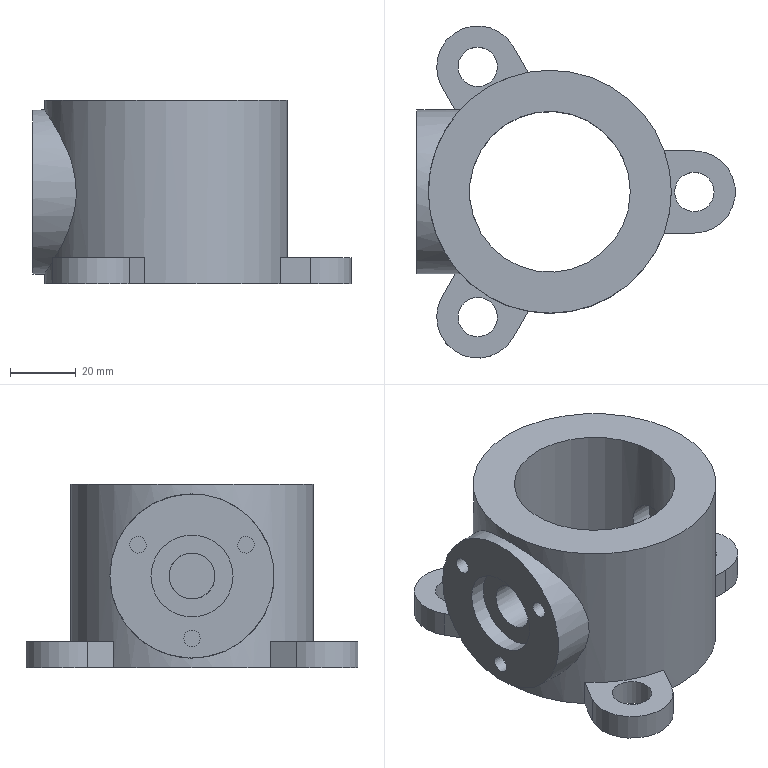Part | NX | features DATUM_CSYS 8, EXTRUDE 7, SKETCH 7 | 1 solid | 32 faces | box 97 x 101.21 x 56 mm | volume 148727 mm3 | plane 17 | cylinder 15 | commonest cylinder face diameters 25 x4 5 x3 12 x3 14 x2 49 x1 50 x1
STEP:
#1=CARTESIAN_POINT('',(-28.238,23.909,8.));
#2=VERTEX_POINT('',#1);
#3=CARTESIAN_POINT('',(-6.587,36.409,8.));
#4=VERTEX_POINT('',#3);
#5=CARTESIAN_POINT('',(0.,0.,8.));
#6=DIRECTION('',(0.,0.,1.));
#7=DIRECTION('',(1.,0.,0.));
#8=AXIS2_PLACEMENT_3D('',#5,#6,#7);
#9=CIRCLE('',#8,37.);
#10=EDGE_CURVE('',#2,#4,#9,.F.);
#11=ORIENTED_EDGE('',*,*,#10,.T.);
#12=CARTESIAN_POINT('',(-11.175,44.355,8.));
#13=VERTEX_POINT('',#12);
#14=CARTESIAN_POINT('',(-6.587,36.409,8.));
#15=DIRECTION('',(-0.5,0.866,0.));
#16=VECTOR('',#15,1000.);
#17=LINE('',#14,#16);
#18=EDGE_CURVE('',#4,#13,#17,.T.);
#19=ORIENTED_EDGE('',*,*,#18,.T.);
#20=CARTESIAN_POINT('',(-32.825,31.855,8.));
#21=VERTEX_POINT('',#20);
#22=CARTESIAN_POINT('',(-22.,38.105,8.));
#23=DIRECTION('',(0.,0.,1.));
#24=DIRECTION('',(-0.5,0.866,0.));
#25=AXIS2_PLACEMENT_3D('',#22,#23,#24);
#26=CIRCLE('',#25,12.5);
#27=EDGE_CURVE('',#13,#21,#26,.T.);
#28=ORIENTED_EDGE('',*,*,#27,.T.);
#29=CARTESIAN_POINT('',(-32.825,31.855,8.));
#30=DIRECTION('',(0.5,-0.866,0.));
#31=VECTOR('',#30,1000.);
#32=LINE('',#29,#31);
#33=EDGE_CURVE('',#21,#2,#32,.T.);
#34=ORIENTED_EDGE('',*,*,#33,.T.);
#35=EDGE_LOOP('',(#11,#19,#28,#34));
#36=FACE_BOUND('',#35,.T.);
#37=CARTESIAN_POINT('',(-25.,43.301,8.));
#38=VERTEX_POINT('',#37);
#39=CARTESIAN_POINT('',(-22.,38.105,8.));
#40=DIRECTION('',(0.,0.,1.));
#41=DIRECTION('',(-0.5,0.866,0.));
#42=AXIS2_PLACEMENT_3D('',#39,#40,#41);
#43=CIRCLE('',#42,6.);
#44=EDGE_CURVE('',#38,#38,#43,.T.);
#45=ORIENTED_EDGE('',*,*,#44,.F.);
#46=EDGE_LOOP('',(#45));
#47=FACE_BOUND('',#46,.T.);
#48=CARTESIAN_POINT('',(-22.,-38.105,8.));
#49=DIRECTION('',(0.,0.,1.));
#50=DIRECTION('',(1.,0.,0.));
#51=AXIS2_PLACEMENT_3D('',#48,#49,#50);
#52=PLANE('',#51);
#53=ADVANCED_FACE('',(#36,#47),#52,.T.);
#54=CARTESIAN_POINT('',(-6.587,-36.409,8.));
#55=VERTEX_POINT('',#54);
#56=CARTESIAN_POINT('',(-28.238,-23.909,8.));
#57=VERTEX_POINT('',#56);
#58=CARTESIAN_POINT('',(0.,0.,8.));
#59=DIRECTION('',(0.,0.,1.));
#60=DIRECTION('',(1.,0.,0.));
#61=AXIS2_PLACEMENT_3D('',#58,#59,#60);
#62=CIRCLE('',#61,37.);
#63=EDGE_CURVE('',#55,#57,#62,.F.);
#64=ORIENTED_EDGE('',*,*,#63,.T.);
#65=CARTESIAN_POINT('',(-32.825,-31.855,8.));
#66=VERTEX_POINT('',#65);
#67=CARTESIAN_POINT('',(-28.238,-23.909,8.));
#68=DIRECTION('',(-0.5,-0.866,0.));
#69=VECTOR('',#68,1000.);
#70=LINE('',#67,#69);
#71=EDGE_CURVE('',#57,#66,#70,.T.);
#72=ORIENTED_EDGE('',*,*,#71,.T.);
#73=CARTESIAN_POINT('',(-11.175,-44.355,8.));
#74=VERTEX_POINT('',#73);
#75=CARTESIAN_POINT('',(-22.,-38.105,8.));
#76=DIRECTION('',(0.,0.,1.));
#77=DIRECTION('',(-0.5,-0.866,0.));
#78=AXIS2_PLACEMENT_3D('',#75,#76,#77);
#79=CIRCLE('',#78,12.5);
#80=EDGE_CURVE('',#66,#74,#79,.T.);
#81=ORIENTED_EDGE('',*,*,#80,.T.);
#82=CARTESIAN_POINT('',(-11.175,-44.355,8.));
#83=DIRECTION('',(0.5,0.866,0.));
#84=VECTOR('',#83,1000.);
#85=LINE('',#82,#84);
#86=EDGE_CURVE('',#74,#55,#85,.T.);
#87=ORIENTED_EDGE('',*,*,#86,.T.);
#88=EDGE_LOOP('',(#64,#72,#81,#87));
#89=FACE_BOUND('',#88,.T.);
#90=CARTESIAN_POINT('',(-25.,-43.301,8.));
#91=VERTEX_POINT('',#90);
#92=CARTESIAN_POINT('',(-22.,-38.105,8.));
#93=DIRECTION('',(0.,0.,1.));
#94=DIRECTION('',(-0.5,-0.866,0.));
#95=AXIS2_PLACEMENT_3D('',#92,#93,#94);
#96=CIRCLE('',#95,6.);
#97=EDGE_CURVE('',#91,#91,#96,.T.);
#98=ORIENTED_EDGE('',*,*,#97,.F.);
#99=EDGE_LOOP('',(#98));
#100=FACE_BOUND('',#99,.T.);
#101=CARTESIAN_POINT('',(-22.,-38.105,8.));
#102=DIRECTION('',(0.,0.,1.));
#103=DIRECTION('',(1.,0.,0.));
#104=AXIS2_PLACEMENT_3D('',#101,#102,#103);
#105=PLANE('',#104);
#106=ADVANCED_FACE('',(#89,#100),#105,.T.);
#107=CARTESIAN_POINT('',(-28.238,-23.909,0.));
#108=VERTEX_POINT('',#107);
#109=CARTESIAN_POINT('',(-32.825,-31.855,0.));
#110=VERTEX_POINT('',#109);
#111=CARTESIAN_POINT('',(-28.238,-23.909,0.));
#112=DIRECTION('',(-0.5,-0.866,0.));
#113=VECTOR('',#112,1000.);
#114=LINE('',#111,#113);
#115=EDGE_CURVE('',#108,#110,#114,.T.);
#116=ORIENTED_EDGE('',*,*,#115,.T.);
#117=CARTESIAN_POINT('',(-32.825,-31.855,8.));
#118=DIRECTION('',(0.,0.,-1.));
#119=VECTOR('',#118,1000.);
#120=LINE('',#117,#119);
#121=EDGE_CURVE('',#66,#110,#120,.T.);
#122=ORIENTED_EDGE('',*,*,#121,.F.);
#123=ORIENTED_EDGE('',*,*,#71,.F.);
#124=CARTESIAN_POINT('',(-28.238,-23.909,8.));
#125=DIRECTION('',(0.,0.,-1.));
#126=VECTOR('',#125,1000.);
#127=LINE('',#124,#126);
#128=EDGE_CURVE('',#57,#108,#127,.T.);
#129=ORIENTED_EDGE('',*,*,#128,.T.);
#130=EDGE_LOOP('',(#116,#122,#123,#129));
#131=FACE_BOUND('',#130,.T.);
#132=CARTESIAN_POINT('',(-28.238,-23.909,8.));
#133=DIRECTION('',(0.866,-0.5,0.));
#134=DIRECTION('',(0.5,0.866,0.));
#135=AXIS2_PLACEMENT_3D('',#132,#133,#134);
#136=PLANE('',#135);
#137=ADVANCED_FACE('',(#131),#136,.F.);
#138=CARTESIAN_POINT('',(-11.175,-44.355,0.));
#139=VERTEX_POINT('',#138);
#140=CARTESIAN_POINT('',(-22.,-38.105,0.));
#141=DIRECTION('',(0.,0.,1.));
#142=DIRECTION('',(-0.5,-0.866,0.));
#143=AXIS2_PLACEMENT_3D('',#140,#141,#142);
#144=CIRCLE('',#143,12.5);
#145=EDGE_CURVE('',#110,#139,#144,.T.);
#146=ORIENTED_EDGE('',*,*,#145,.T.);
#147=CARTESIAN_POINT('',(-11.175,-44.355,8.));
#148=DIRECTION('',(0.,0.,-1.));
#149=VECTOR('',#148,1000.);
#150=LINE('',#147,#149);
#151=EDGE_CURVE('',#74,#139,#150,.T.);
#152=ORIENTED_EDGE('',*,*,#151,.F.);
#153=ORIENTED_EDGE('',*,*,#80,.F.);
#154=ORIENTED_EDGE('',*,*,#121,.T.);
#155=EDGE_LOOP('',(#146,#152,#153,#154));
#156=FACE_BOUND('',#155,.T.);
#157=CARTESIAN_POINT('',(-22.,-38.105,8.));
#158=DIRECTION('',(0.,0.,-1.));
#159=DIRECTION('',(-1.,0.,0.));
#160=AXIS2_PLACEMENT_3D('',#157,#158,#159);
#161=CYLINDRICAL_SURFACE('',#160,12.5);
#162=ADVANCED_FACE('',(#156),#161,.T.);
#163=CARTESIAN_POINT('',(-6.587,-36.409,0.));
#164=VERTEX_POINT('',#163);
#165=CARTESIAN_POINT('',(-11.175,-44.355,0.));
#166=DIRECTION('',(0.5,0.866,0.));
#167=VECTOR('',#166,1000.);
#168=LINE('',#165,#167);
#169=EDGE_CURVE('',#139,#164,#168,.T.);
#170=ORIENTED_EDGE('',*,*,#169,.T.);
#171=CARTESIAN_POINT('',(-6.587,-36.409,8.));
#172=DIRECTION('',(0.,0.,-1.));
#173=VECTOR('',#172,1000.);
#174=LINE('',#171,#173);
#175=EDGE_CURVE('',#55,#164,#174,.T.);
#176=ORIENTED_EDGE('',*,*,#175,.F.);
#177=ORIENTED_EDGE('',*,*,#86,.F.);
#178=ORIENTED_EDGE('',*,*,#151,.T.);
#179=EDGE_LOOP('',(#170,#176,#177,#178));
#180=FACE_BOUND('',#179,.T.);
#181=CARTESIAN_POINT('',(-11.175,-44.355,8.));
#182=DIRECTION('',(-0.866,0.5,0.));
#183=DIRECTION('',(-0.5,-0.866,0.));
#184=AXIS2_PLACEMENT_3D('',#181,#182,#183);
#185=PLANE('',#184);
#186=ADVANCED_FACE('',(#180),#185,.F.);
#187=CARTESIAN_POINT('',(34.825,-12.5,0.));
#188=VERTEX_POINT('',#187);
#189=CARTESIAN_POINT('',(44.,-12.5,0.));
#190=VERTEX_POINT('',#189);
#191=CARTESIAN_POINT('',(34.825,-12.5,0.));
#192=DIRECTION('',(1.,0.,0.));
#193=VECTOR('',#192,1000.);
#194=LINE('',#191,#193);
#195=EDGE_CURVE('',#188,#190,#194,.T.);
#196=ORIENTED_EDGE('',*,*,#195,.T.);
#197=CARTESIAN_POINT('',(44.,-12.5,8.));
#198=VERTEX_POINT('',#197);
#199=CARTESIAN_POINT('',(44.,-12.5,8.));
#200=DIRECTION('',(0.,0.,-1.));
#201=VECTOR('',#200,1000.);
#202=LINE('',#199,#201);
#203=EDGE_CURVE('',#198,#190,#202,.T.);
#204=ORIENTED_EDGE('',*,*,#203,.F.);
#205=CARTESIAN_POINT('',(34.825,-12.5,8.));
#206=VERTEX_POINT('',#205);
#207=CARTESIAN_POINT('',(34.825,-12.5,8.));
#208=DIRECTION('',(1.,0.,0.));
#209=VECTOR('',#208,1000.);
#210=LINE('',#207,#209);
#211=EDGE_CURVE('',#206,#198,#210,.T.);
#212=ORIENTED_EDGE('',*,*,#211,.F.);
#213=CARTESIAN_POINT('',(34.825,-12.5,8.));
#214=DIRECTION('',(0.,0.,-1.));
#215=VECTOR('',#214,1000.);
#216=LINE('',#213,#215);
#217=EDGE_CURVE('',#206,#188,#216,.T.);
#218=ORIENTED_EDGE('',*,*,#217,.T.);
#219=EDGE_LOOP('',(#196,#204,#212,#218));
#220=FACE_BOUND('',#219,.T.);
#221=CARTESIAN_POINT('',(34.825,-12.5,8.));
#222=DIRECTION('',(0.,1.,0.));
#223=DIRECTION('',(-1.,0.,0.));
#224=AXIS2_PLACEMENT_3D('',#221,#222,#223);
#225=PLANE('',#224);
#226=ADVANCED_FACE('',(#220),#225,.F.);
#227=CARTESIAN_POINT('',(44.,12.5,0.));
#228=VERTEX_POINT('',#227);
#229=CARTESIAN_POINT('',(44.,0.,0.));
#230=DIRECTION('',(0.,0.,1.));
#231=DIRECTION('',(1.,0.,0.));
#232=AXIS2_PLACEMENT_3D('',#229,#230,#231);
#233=CIRCLE('',#232,12.5);
#234=EDGE_CURVE('',#190,#228,#233,.T.);
#235=ORIENTED_EDGE('',*,*,#234,.T.);
#236=CARTESIAN_POINT('',(44.,12.5,8.));
#237=VERTEX_POINT('',#236);
#238=CARTESIAN_POINT('',(44.,12.5,8.));
#239=DIRECTION('',(0.,0.,-1.));
#240=VECTOR('',#239,1000.);
#241=LINE('',#238,#240);
#242=EDGE_CURVE('',#237,#228,#241,.T.);
#243=ORIENTED_EDGE('',*,*,#242,.F.);
#244=CARTESIAN_POINT('',(44.,0.,8.));
#245=DIRECTION('',(0.,0.,1.));
#246=DIRECTION('',(1.,0.,0.));
#247=AXIS2_PLACEMENT_3D('',#244,#245,#246);
#248=CIRCLE('',#247,12.5);
#249=EDGE_CURVE('',#198,#237,#248,.T.);
#250=ORIENTED_EDGE('',*,*,#249,.F.);
#251=ORIENTED_EDGE('',*,*,#203,.T.);
#252=EDGE_LOOP('',(#235,#243,#250,#251));
#253=FACE_BOUND('',#252,.T.);
#254=CARTESIAN_POINT('',(44.,0.,8.));
#255=DIRECTION('',(0.,0.,-1.));
#256=DIRECTION('',(-1.,0.,0.));
#257=AXIS2_PLACEMENT_3D('',#254,#255,#256);
#258=CYLINDRICAL_SURFACE('',#257,12.5);
#259=ADVANCED_FACE('',(#253),#258,.T.);
#260=CARTESIAN_POINT('',(34.825,12.5,0.));
#261=VERTEX_POINT('',#260);
#262=CARTESIAN_POINT('',(44.,12.5,0.));
#263=DIRECTION('',(-1.,0.,0.));
#264=VECTOR('',#263,1000.);
#265=LINE('',#262,#264);
#266=EDGE_CURVE('',#228,#261,#265,.T.);
#267=ORIENTED_EDGE('',*,*,#266,.T.);
#268=CARTESIAN_POINT('',(34.825,12.5,8.));
#269=VERTEX_POINT('',#268);
#270=CARTESIAN_POINT('',(34.825,12.5,8.));
#271=DIRECTION('',(0.,0.,-1.));
#272=VECTOR('',#271,1000.);
#273=LINE('',#270,#272);
#274=EDGE_CURVE('',#269,#261,#273,.T.);
#275=ORIENTED_EDGE('',*,*,#274,.F.);
#276=CARTESIAN_POINT('',(44.,12.5,8.));
#277=DIRECTION('',(-1.,0.,0.));
#278=VECTOR('',#277,1000.);
#279=LINE('',#276,#278);
#280=EDGE_CURVE('',#237,#269,#279,.T.);
#281=ORIENTED_EDGE('',*,*,#280,.F.);
#282=ORIENTED_EDGE('',*,*,#242,.T.);
#283=EDGE_LOOP('',(#267,#275,#281,#282));
#284=FACE_BOUND('',#283,.T.);
#285=CARTESIAN_POINT('',(44.,12.5,8.));
#286=DIRECTION('',(0.,-1.,0.));
#287=DIRECTION('',(1.,0.,0.));
#288=AXIS2_PLACEMENT_3D('',#285,#286,#287);
#289=PLANE('',#288);
#290=ADVANCED_FACE('',(#284),#289,.F.);
#291=CARTESIAN_POINT('',(-6.587,36.409,0.));
#292=VERTEX_POINT('',#291);
#293=CARTESIAN_POINT('',(-11.175,44.355,0.));
#294=VERTEX_POINT('',#293);
#295=CARTESIAN_POINT('',(-6.587,36.409,0.));
#296=DIRECTION('',(-0.5,0.866,0.));
#297=VECTOR('',#296,1000.);
#298=LINE('',#295,#297);
#299=EDGE_CURVE('',#292,#294,#298,.T.);
#300=ORIENTED_EDGE('',*,*,#299,.T.);
#301=CARTESIAN_POINT('',(-11.175,44.355,8.));
#302=DIRECTION('',(0.,0.,-1.));
#303=VECTOR('',#302,1000.);
#304=LINE('',#301,#303);
#305=EDGE_CURVE('',#13,#294,#304,.T.);
#306=ORIENTED_EDGE('',*,*,#305,.F.);
#307=ORIENTED_EDGE('',*,*,#18,.F.);
#308=CARTESIAN_POINT('',(-6.587,36.409,8.));
#309=DIRECTION('',(0.,0.,-1.));
#310=VECTOR('',#309,1000.);
#311=LINE('',#308,#310);
#312=EDGE_CURVE('',#4,#292,#311,.T.);
#313=ORIENTED_EDGE('',*,*,#312,.T.);
#314=EDGE_LOOP('',(#300,#306,#307,#313));
#315=FACE_BOUND('',#314,.T.);
#316=CARTESIAN_POINT('',(-6.587,36.409,8.));
#317=DIRECTION('',(-0.866,-0.5,0.));
#318=DIRECTION('',(0.5,-0.866,0.));
#319=AXIS2_PLACEMENT_3D('',#316,#317,#318);
#320=PLANE('',#319);
#321=ADVANCED_FACE('',(#315),#320,.F.);
#322=CARTESIAN_POINT('',(-32.825,31.855,0.));
#323=VERTEX_POINT('',#322);
#324=CARTESIAN_POINT('',(-22.,38.105,0.));
#325=DIRECTION('',(0.,0.,1.));
#326=DIRECTION('',(-0.5,0.866,0.));
#327=AXIS2_PLACEMENT_3D('',#324,#325,#326);
#328=CIRCLE('',#327,12.5);
#329=EDGE_CURVE('',#294,#323,#328,.T.);
#330=ORIENTED_EDGE('',*,*,#329,.T.);
#331=CARTESIAN_POINT('',(-32.825,31.855,8.));
#332=DIRECTION('',(0.,0.,-1.));
#333=VECTOR('',#332,1000.);
#334=LINE('',#331,#333);
#335=EDGE_CURVE('',#21,#323,#334,.T.);
#336=ORIENTED_EDGE('',*,*,#335,.F.);
#337=ORIENTED_EDGE('',*,*,#27,.F.);
#338=ORIENTED_EDGE('',*,*,#305,.T.);
#339=EDGE_LOOP('',(#330,#336,#337,#338));
#340=FACE_BOUND('',#339,.T.);
#341=CARTESIAN_POINT('',(-22.,38.105,8.));
#342=DIRECTION('',(0.,0.,-1.));
#343=DIRECTION('',(-1.,0.,0.));
#344=AXIS2_PLACEMENT_3D('',#341,#342,#343);
#345=CYLINDRICAL_SURFACE('',#344,12.5);
#346=ADVANCED_FACE('',(#340),#345,.T.);
#347=CARTESIAN_POINT('',(-28.238,23.909,0.));
#348=VERTEX_POINT('',#347);
#349=CARTESIAN_POINT('',(-32.825,31.855,0.));
#350=DIRECTION('',(0.5,-0.866,0.));
#351=VECTOR('',#350,1000.);
#352=LINE('',#349,#351);
#353=EDGE_CURVE('',#323,#348,#352,.T.);
#354=ORIENTED_EDGE('',*,*,#353,.T.);
#355=CARTESIAN_POINT('',(-28.238,23.909,8.));
#356=DIRECTION('',(0.,0.,-1.));
#357=VECTOR('',#356,1000.);
#358=LINE('',#355,#357);
#359=EDGE_CURVE('',#2,#348,#358,.T.);
#360=ORIENTED_EDGE('',*,*,#359,.F.);
#361=ORIENTED_EDGE('',*,*,#33,.F.);
#362=ORIENTED_EDGE('',*,*,#335,.T.);
#363=EDGE_LOOP('',(#354,#360,#361,#362));
#364=FACE_BOUND('',#363,.T.);
#365=CARTESIAN_POINT('',(-32.825,31.855,8.));
#366=DIRECTION('',(0.866,0.5,0.));
#367=DIRECTION('',(-0.5,0.866,0.));
#368=AXIS2_PLACEMENT_3D('',#365,#366,#367);
#369=PLANE('',#368);
#370=ADVANCED_FACE('',(#364),#369,.F.);
#371=ORIENTED_EDGE('',*,*,#44,.T.);
#372=EDGE_LOOP('',(#371));
#373=FACE_BOUND('',#372,.T.);
#374=CARTESIAN_POINT('',(-25.,43.301,0.));
#375=VERTEX_POINT('',#374);
#376=CARTESIAN_POINT('',(-22.,38.105,0.));
#377=DIRECTION('',(0.,0.,1.));
#378=DIRECTION('',(-0.5,0.866,0.));
#379=AXIS2_PLACEMENT_3D('',#376,#377,#378);
#380=CIRCLE('',#379,6.);
#381=EDGE_CURVE('',#375,#375,#380,.T.);
#382=ORIENTED_EDGE('',*,*,#381,.F.);
#383=EDGE_LOOP('',(#382));
#384=FACE_BOUND('',#383,.T.);
#385=CARTESIAN_POINT('',(-22.,38.105,8.));
#386=DIRECTION('',(0.,0.,-1.));
#387=DIRECTION('',(-1.,0.,0.));
#388=AXIS2_PLACEMENT_3D('',#385,#386,#387);
#389=CYLINDRICAL_SURFACE('',#388,6.);
#390=ADVANCED_FACE('',(#373,#384),#389,.F.);
#391=ORIENTED_EDGE('',*,*,#97,.T.);
#392=EDGE_LOOP('',(#391));
#393=FACE_BOUND('',#392,.T.);
#394=CARTESIAN_POINT('',(-25.,-43.301,0.));
#395=VERTEX_POINT('',#394);
#396=CARTESIAN_POINT('',(-22.,-38.105,0.));
#397=DIRECTION('',(0.,0.,1.));
#398=DIRECTION('',(-0.5,-0.866,0.));
#399=AXIS2_PLACEMENT_3D('',#396,#397,#398);
#400=CIRCLE('',#399,6.);
#401=EDGE_CURVE('',#395,#395,#400,.T.);
#402=ORIENTED_EDGE('',*,*,#401,.F.);
#403=EDGE_LOOP('',(#402));
#404=FACE_BOUND('',#403,.T.);
#405=CARTESIAN_POINT('',(-22.,-38.105,8.));
#406=DIRECTION('',(0.,0.,-1.));
#407=DIRECTION('',(-1.,0.,0.));
#408=AXIS2_PLACEMENT_3D('',#405,#406,#407);
#409=CYLINDRICAL_SURFACE('',#408,6.);
#410=ADVANCED_FACE('',(#393,#404),#409,.F.);
#411=CARTESIAN_POINT('',(-37.,0.,53.));
#412=VERTEX_POINT('',#411);
#413=CARTESIAN_POINT('',(-36.003,10.183,51.555));
#414=CARTESIAN_POINT('',(-37.496,-0.01121,53.72));
#415=CARTESIAN_POINT('',(-36.013,-10.138,51.566));
#416=CARTESIAN_POINT('',(-33.123,-16.821,46.966));
#417=CARTESIAN_POINT('',(-30.616,-20.859,42.049));
#418=CARTESIAN_POINT('',(-28.91,-23.134,37.88));
#419=CARTESIAN_POINT('',(-27.613,-24.641,33.135));
#420=CARTESIAN_POINT('',(-26.937,-25.357,26.333));
#421=CARTESIAN_POINT('',(-28.645,-23.584,17.943));
#422=CARTESIAN_POINT('',(-32.521,-18.205,10.023));
#423=CARTESIAN_POINT('',(-35.988,-10.227,4.464));
#424=CARTESIAN_POINT('',(-37.495,-0.06125,2.284));
#425=CARTESIAN_POINT('',(-36.033,10.083,4.401));
#426=CARTESIAN_POINT('',(-32.547,18.162,9.962));
#427=CARTESIAN_POINT('',(-29.331,22.649,16.575));
#428=CARTESIAN_POINT('',(-27.609,24.643,22.881));
#429=CARTESIAN_POINT('',(-27.112,25.176,27.969));
#430=CARTESIAN_POINT('',(-27.6,24.654,33.077));
#431=CARTESIAN_POINT('',(-29.323,22.66,39.41));
#432=CARTESIAN_POINT('',(-32.538,18.168,46.019));
#433=CARTESIAN_POINT('',(-36.003,10.183,51.555));
#434=CARTESIAN_POINT('',(-37.496,-0.01121,53.72));
#435=CARTESIAN_POINT('',(-36.013,-10.138,51.566));
#436=B_SPLINE_CURVE_WITH_KNOTS('',3,(#413,#414,#415,#416,#417,#418,#419,#420,#421,#422,#423,#424,#425,#426,#427,#428,#429,#430,#431,#432,#433,#434,#435),.UNSPECIFIED.,.T.,.F.,(1,1,1,1,1,1,1,1,1,1,1,1,1,1,1,1,1,1,1,1,1,1,1,1,1,1,1),(-0.03032,-0.02021,-0.01011,0.,0.01011,0.02021,0.02527,0.03032,0.03537,0.04043,0.05054,0.06064,0.07075,0.08086,0.09096,0.1011,0.1112,0.1162,0.1213,0.1263,0.1314,0.1415,0.1516,0.1617,0.1718,0.1819,0.187),.UNSPECIFIED.);
#437=EDGE_CURVE('',#412,#412,#436,.T.);
#438=ORIENTED_EDGE('',*,*,#437,.T.);
#439=EDGE_LOOP('',(#438));
#440=FACE_BOUND('',#439,.T.);
#441=CARTESIAN_POINT('',(0.,0.,0.));
#442=DIRECTION('',(0.,0.,1.));
#443=DIRECTION('',(1.,0.,0.));
#444=AXIS2_PLACEMENT_3D('',#441,#442,#443);
#445=CIRCLE('',#444,37.);
#446=EDGE_CURVE('',#348,#108,#445,.T.);
#447=ORIENTED_EDGE('',*,*,#446,.T.);
#448=ORIENTED_EDGE('',*,*,#128,.F.);
#449=ORIENTED_EDGE('',*,*,#63,.F.);
#450=ORIENTED_EDGE('',*,*,#175,.T.);
#451=CARTESIAN_POINT('',(0.,0.,0.));
#452=DIRECTION('',(0.,0.,1.));
#453=DIRECTION('',(1.,0.,0.));
#454=AXIS2_PLACEMENT_3D('',#451,#452,#453);
#455=CIRCLE('',#454,37.);
#456=EDGE_CURVE('',#164,#188,#455,.T.);
#457=ORIENTED_EDGE('',*,*,#456,.T.);
#458=ORIENTED_EDGE('',*,*,#217,.F.);
#459=CARTESIAN_POINT('',(0.,0.,8.));
#460=DIRECTION('',(0.,0.,1.));
#461=DIRECTION('',(1.,0.,0.));
#462=AXIS2_PLACEMENT_3D('',#459,#460,#461);
#463=CIRCLE('',#462,37.);
#464=EDGE_CURVE('',#269,#206,#463,.F.);
#465=ORIENTED_EDGE('',*,*,#464,.F.);
#466=ORIENTED_EDGE('',*,*,#274,.T.);
#467=CARTESIAN_POINT('',(0.,0.,0.));
#468=DIRECTION('',(0.,0.,1.));
#469=DIRECTION('',(1.,0.,0.));
#470=AXIS2_PLACEMENT_3D('',#467,#468,#469);
#471=CIRCLE('',#470,37.);
#472=EDGE_CURVE('',#261,#292,#471,.T.);
#473=ORIENTED_EDGE('',*,*,#472,.T.);
#474=ORIENTED_EDGE('',*,*,#312,.F.);
#475=ORIENTED_EDGE('',*,*,#10,.F.);
#476=ORIENTED_EDGE('',*,*,#359,.T.);
#477=EDGE_LOOP('',(#447,#448,#449,#450,#457,#458,#465,#466,#473,#474,#475,#476));
#478=FACE_BOUND('',#477,.T.);
#479=CARTESIAN_POINT('',(37.,0.,56.));
#480=VERTEX_POINT('',#479);
#481=CARTESIAN_POINT('',(0.,0.,56.));
#482=DIRECTION('',(0.,0.,-1.));
#483=DIRECTION('',(1.,0.,0.));
#484=AXIS2_PLACEMENT_3D('',#481,#482,#483);
#485=CIRCLE('',#484,37.);
#486=EDGE_CURVE('',#480,#480,#485,.T.);
#487=ORIENTED_EDGE('',*,*,#486,.T.);
#488=EDGE_LOOP('',(#487));
#489=FACE_BOUND('',#488,.T.);
#490=CARTESIAN_POINT('',(0.,0.,8.));
#491=DIRECTION('',(0.,0.,-1.));
#492=DIRECTION('',(-1.,0.,0.));
#493=AXIS2_PLACEMENT_3D('',#490,#491,#492);
#494=CYLINDRICAL_SURFACE('',#493,37.);
#495=ADVANCED_FACE('',(#440,#478,#489),#494,.T.);
#496=CARTESIAN_POINT('',(50.,0.,8.));
#497=VERTEX_POINT('',#496);
#498=CARTESIAN_POINT('',(44.,0.,8.));
#499=DIRECTION('',(0.,0.,1.));
#500=DIRECTION('',(1.,0.,0.));
#501=AXIS2_PLACEMENT_3D('',#498,#499,#500);
#502=CIRCLE('',#501,6.);
#503=EDGE_CURVE('',#497,#497,#502,.T.);
#504=ORIENTED_EDGE('',*,*,#503,.T.);
#505=EDGE_LOOP('',(#504));
#506=FACE_BOUND('',#505,.T.);
#507=CARTESIAN_POINT('',(50.,0.,0.));
#508=VERTEX_POINT('',#507);
#509=CARTESIAN_POINT('',(44.,0.,0.));
#510=DIRECTION('',(0.,0.,1.));
#511=DIRECTION('',(1.,0.,0.));
#512=AXIS2_PLACEMENT_3D('',#509,#510,#511);
#513=CIRCLE('',#512,6.);
#514=EDGE_CURVE('',#508,#508,#513,.T.);
#515=ORIENTED_EDGE('',*,*,#514,.F.);
#516=EDGE_LOOP('',(#515));
#517=FACE_BOUND('',#516,.T.);
#518=CARTESIAN_POINT('',(44.,0.,8.));
#519=DIRECTION('',(0.,0.,-1.));
#520=DIRECTION('',(-1.,0.,0.));
#521=AXIS2_PLACEMENT_3D('',#518,#519,#520);
#522=CYLINDRICAL_SURFACE('',#521,6.);
#523=ADVANCED_FACE('',(#506,#517),#522,.F.);
#524=ORIENTED_EDGE('',*,*,#464,.T.);
#525=ORIENTED_EDGE('',*,*,#211,.T.);
#526=ORIENTED_EDGE('',*,*,#249,.T.);
#527=ORIENTED_EDGE('',*,*,#280,.T.);
#528=EDGE_LOOP('',(#524,#525,#526,#527));
#529=FACE_BOUND('',#528,.T.);
#530=ORIENTED_EDGE('',*,*,#503,.F.);
#531=EDGE_LOOP('',(#530));
#532=FACE_BOUND('',#531,.T.);
#533=CARTESIAN_POINT('',(-22.,-38.105,8.));
#534=DIRECTION('',(0.,0.,1.));
#535=DIRECTION('',(1.,0.,0.));
#536=AXIS2_PLACEMENT_3D('',#533,#534,#535);
#537=PLANE('',#536);
#538=ADVANCED_FACE('',(#529,#532),#537,.T.);
#539=CARTESIAN_POINT('',(24.5,0.,0.));
#540=VERTEX_POINT('',#539);
#541=CARTESIAN_POINT('',(0.,0.,0.));
#542=DIRECTION('',(0.,0.,1.));
#543=DIRECTION('',(1.,0.,0.));
#544=AXIS2_PLACEMENT_3D('',#541,#542,#543);
#545=CIRCLE('',#544,24.5);
#546=EDGE_CURVE('',#540,#540,#545,.T.);
#547=ORIENTED_EDGE('',*,*,#546,.T.);
#548=EDGE_LOOP('',(#547));
#549=FACE_BOUND('',#548,.T.);
#550=ORIENTED_EDGE('',*,*,#195,.F.);
#551=ORIENTED_EDGE('',*,*,#456,.F.);
#552=ORIENTED_EDGE('',*,*,#169,.F.);
#553=ORIENTED_EDGE('',*,*,#145,.F.);
#554=ORIENTED_EDGE('',*,*,#115,.F.);
#555=ORIENTED_EDGE('',*,*,#446,.F.);
#556=ORIENTED_EDGE('',*,*,#353,.F.);
#557=ORIENTED_EDGE('',*,*,#329,.F.);
#558=ORIENTED_EDGE('',*,*,#299,.F.);
#559=ORIENTED_EDGE('',*,*,#472,.F.);
#560=ORIENTED_EDGE('',*,*,#266,.F.);
#561=ORIENTED_EDGE('',*,*,#234,.F.);
#562=EDGE_LOOP('',(#550,#551,#552,#553,#554,#555,#556,#557,#558,#559,#560,#561));
#563=FACE_BOUND('',#562,.T.);
#564=ORIENTED_EDGE('',*,*,#514,.T.);
#565=EDGE_LOOP('',(#564));
#566=FACE_BOUND('',#565,.T.);
#567=ORIENTED_EDGE('',*,*,#381,.T.);
#568=EDGE_LOOP('',(#567));
#569=FACE_BOUND('',#568,.T.);
#570=ORIENTED_EDGE('',*,*,#401,.T.);
#571=EDGE_LOOP('',(#570));
#572=FACE_BOUND('',#571,.T.);
#573=CARTESIAN_POINT('',(-22.,-38.105,0.));
#574=DIRECTION('',(0.,0.,1.));
#575=DIRECTION('',(1.,0.,0.));
#576=AXIS2_PLACEMENT_3D('',#573,#574,#575);
#577=PLANE('',#576);
#578=ADVANCED_FACE('',(#549,#563,#566,#569,#572),#577,.F.);
#579=CARTESIAN_POINT('',(24.5,0.,56.));
#580=VERTEX_POINT('',#579);
#581=CARTESIAN_POINT('',(0.,0.,56.));
#582=DIRECTION('',(0.,0.,1.));
#583=DIRECTION('',(1.,0.,0.));
#584=AXIS2_PLACEMENT_3D('',#581,#582,#583);
#585=CIRCLE('',#584,24.5);
#586=EDGE_CURVE('',#580,#580,#585,.T.);
#587=ORIENTED_EDGE('',*,*,#586,.F.);
#588=EDGE_LOOP('',(#587));
#589=FACE_BOUND('',#588,.T.);
#590=ORIENTED_EDGE('',*,*,#486,.F.);
#591=EDGE_LOOP('',(#590));
#592=FACE_BOUND('',#591,.T.);
#593=CARTESIAN_POINT('',(0.,0.,56.));
#594=DIRECTION('',(0.,0.,-1.));
#595=DIRECTION('',(-1.,0.,0.));
#596=AXIS2_PLACEMENT_3D('',#593,#594,#595);
#597=PLANE('',#596);
#598=ADVANCED_FACE('',(#589,#592),#597,.F.);
#599=CARTESIAN_POINT('',(-40.5,25.,28.));
#600=VERTEX_POINT('',#599);
#601=CARTESIAN_POINT('',(-40.5,0.,28.));
#602=DIRECTION('',(1.,0.,0.));
#603=DIRECTION('',(0.,1.,0.));
#604=AXIS2_PLACEMENT_3D('',#601,#602,#603);
#605=CIRCLE('',#604,25.);
#606=EDGE_CURVE('',#600,#600,#605,.T.);
#607=ORIENTED_EDGE('',*,*,#606,.T.);
#608=EDGE_LOOP('',(#607));
#609=FACE_BOUND('',#608,.T.);
#610=ORIENTED_EDGE('',*,*,#437,.F.);
#611=EDGE_LOOP('',(#610));
#612=FACE_BOUND('',#611,.T.);
#613=CARTESIAN_POINT('',(-40.5,0.,28.));
#614=DIRECTION('',(1.,0.,0.));
#615=DIRECTION('',(0.,0.,-1.));
#616=AXIS2_PLACEMENT_3D('',#613,#614,#615);
#617=CYLINDRICAL_SURFACE('',#616,25.);
#618=ADVANCED_FACE('',(#609,#612),#617,.T.);
#619=CARTESIAN_POINT('',(-40.5,12.5,28.));
#620=VERTEX_POINT('',#619);
#621=CARTESIAN_POINT('',(-40.5,0.,28.));
#622=DIRECTION('',(-1.,0.,0.));
#623=DIRECTION('',(0.,1.,0.));
#624=AXIS2_PLACEMENT_3D('',#621,#622,#623);
#625=CIRCLE('',#624,12.5);
#626=EDGE_CURVE('',#620,#620,#625,.T.);
#627=ORIENTED_EDGE('',*,*,#626,.F.);
#628=EDGE_LOOP('',(#627));
#629=FACE_BOUND('',#628,.T.);
#630=CARTESIAN_POINT('',(-40.5,2.5,9.));
#631=VERTEX_POINT('',#630);
#632=CARTESIAN_POINT('',(-40.5,0.,9.));
#633=DIRECTION('',(-1.,0.,0.));
#634=DIRECTION('',(0.,1.,0.));
#635=AXIS2_PLACEMENT_3D('',#632,#633,#634);
#636=CIRCLE('',#635,2.5);
#637=EDGE_CURVE('',#631,#631,#636,.T.);
#638=ORIENTED_EDGE('',*,*,#637,.F.);
#639=EDGE_LOOP('',(#638));
#640=FACE_BOUND('',#639,.T.);
#641=CARTESIAN_POINT('',(-40.5,-17.704,35.335));
#642=VERTEX_POINT('',#641);
#643=CARTESIAN_POINT('',(-40.5,-16.454,37.5));
#644=DIRECTION('',(-1.,0.,0.));
#645=DIRECTION('',(0.,-0.5,-0.866));
#646=AXIS2_PLACEMENT_3D('',#643,#644,#645);
#647=CIRCLE('',#646,2.5);
#648=EDGE_CURVE('',#642,#642,#647,.T.);
#649=ORIENTED_EDGE('',*,*,#648,.F.);
#650=EDGE_LOOP('',(#649));
#651=FACE_BOUND('',#650,.T.);
#652=CARTESIAN_POINT('',(-40.5,15.204,39.665));
#653=VERTEX_POINT('',#652);
#654=CARTESIAN_POINT('',(-40.5,16.454,37.5));
#655=DIRECTION('',(-1.,0.,0.));
#656=DIRECTION('',(0.,-0.5,0.866));
#657=AXIS2_PLACEMENT_3D('',#654,#655,#656);
#658=CIRCLE('',#657,2.5);
#659=EDGE_CURVE('',#653,#653,#658,.T.);
#660=ORIENTED_EDGE('',*,*,#659,.F.);
#661=EDGE_LOOP('',(#660));
#662=FACE_BOUND('',#661,.T.);
#663=ORIENTED_EDGE('',*,*,#606,.F.);
#664=EDGE_LOOP('',(#663));
#665=FACE_BOUND('',#664,.T.);
#666=CARTESIAN_POINT('',(-40.5,0.,28.));
#667=DIRECTION('',(1.,0.,0.));
#668=DIRECTION('',(0.,0.,-1.));
#669=AXIS2_PLACEMENT_3D('',#666,#667,#668);
#670=PLANE('',#669);
#671=ADVANCED_FACE('',(#629,#640,#651,#662,#665),#670,.F.);
#672=CARTESIAN_POINT('',(24.5,0.,21.));
#673=VERTEX_POINT('',#672);
#674=CARTESIAN_POINT('',(23.999,-5.49,22.519));
#675=CARTESIAN_POINT('',(24.75,0.000685,20.24));
#676=CARTESIAN_POINT('',(24.,5.487,22.519));
#677=CARTESIAN_POINT('',(23.218,7.757,27.991));
#678=CARTESIAN_POINT('',(24.,5.484,33.488));
#679=CARTESIAN_POINT('',(24.75,0.003958,35.756));
#680=CARTESIAN_POINT('',(24.001,-5.482,33.489));
#681=CARTESIAN_POINT('',(23.218,-7.757,28.002));
#682=CARTESIAN_POINT('',(23.999,-5.49,22.519));
#683=CARTESIAN_POINT('',(24.75,0.000685,20.24));
#684=CARTESIAN_POINT('',(24.,5.487,22.519));
#685=B_SPLINE_CURVE_WITH_KNOTS('',3,(#674,#675,#676,#677,#678,#679,#680,#681,#682,#683,#684),.UNSPECIFIED.,.T.,.F.,(1,1,1,1,1,1,1,1,1,1,1,1,1,1,1),(-0.0165,-0.011,-0.005499,0.,0.005499,0.011,0.0165,0.022,0.0275,0.033,0.0385,0.04399,0.04949,0.05499,0.06049),.UNSPECIFIED.);
#686=EDGE_CURVE('',#673,#673,#685,.T.);
#687=ORIENTED_EDGE('',*,*,#686,.T.);
#688=EDGE_LOOP('',(#687));
#689=FACE_BOUND('',#688,.T.);
#690=CARTESIAN_POINT('',(-24.5,0.,35.));
#691=VERTEX_POINT('',#690);
#692=CARTESIAN_POINT('',(-23.999,-5.49,33.481));
#693=CARTESIAN_POINT('',(-24.75,0.000685,35.76));
#694=CARTESIAN_POINT('',(-24.,5.487,33.481));
#695=CARTESIAN_POINT('',(-23.218,7.757,28.009));
#696=CARTESIAN_POINT('',(-24.,5.484,22.512));
#697=CARTESIAN_POINT('',(-24.75,0.003958,20.244));
#698=CARTESIAN_POINT('',(-24.001,-5.482,22.511));
#699=CARTESIAN_POINT('',(-23.218,-7.757,27.998));
#700=CARTESIAN_POINT('',(-23.999,-5.49,33.481));
#701=CARTESIAN_POINT('',(-24.75,0.000685,35.76));
#702=CARTESIAN_POINT('',(-24.,5.487,33.481));
#703=B_SPLINE_CURVE_WITH_KNOTS('',3,(#692,#693,#694,#695,#696,#697,#698,#699,#700,#701,#702),.UNSPECIFIED.,.T.,.F.,(1,1,1,1,1,1,1,1,1,1,1,1,1,1,1),(-0.0165,-0.011,-0.005499,0.,0.005499,0.011,0.0165,0.022,0.0275,0.033,0.0385,0.04399,0.04949,0.05499,0.06049),.UNSPECIFIED.);
#704=EDGE_CURVE('',#691,#691,#703,.T.);
#705=ORIENTED_EDGE('',*,*,#704,.T.);
#706=EDGE_LOOP('',(#705));
#707=FACE_BOUND('',#706,.T.);
#708=ORIENTED_EDGE('',*,*,#586,.T.);
#709=EDGE_LOOP('',(#708));
#710=FACE_BOUND('',#709,.T.);
#711=ORIENTED_EDGE('',*,*,#546,.F.);
#712=EDGE_LOOP('',(#711));
#713=FACE_BOUND('',#712,.T.);
#714=CARTESIAN_POINT('',(0.,0.,-40.));
#715=DIRECTION('',(0.,0.,1.));
#716=DIRECTION('',(1.,0.,0.));
#717=AXIS2_PLACEMENT_3D('',#714,#715,#716);
#718=CYLINDRICAL_SURFACE('',#717,24.5);
#719=ADVANCED_FACE('',(#689,#707,#710,#713),#718,.F.);
#720=CARTESIAN_POINT('',(-32.5,15.204,39.665));
#721=VERTEX_POINT('',#720);
#722=CARTESIAN_POINT('',(-32.5,16.454,37.5));
#723=DIRECTION('',(-1.,0.,0.));
#724=DIRECTION('',(0.,-0.5,0.866));
#725=AXIS2_PLACEMENT_3D('',#722,#723,#724);
#726=CIRCLE('',#725,2.5);
#727=EDGE_CURVE('',#721,#721,#726,.F.);
#728=ORIENTED_EDGE('',*,*,#727,.T.);
#729=EDGE_LOOP('',(#728));
#730=FACE_BOUND('',#729,.T.);
#731=ORIENTED_EDGE('',*,*,#659,.T.);
#732=EDGE_LOOP('',(#731));
#733=FACE_BOUND('',#732,.T.);
#734=CARTESIAN_POINT('',(-32.5,16.454,37.5));
#735=DIRECTION('',(-1.,0.,0.));
#736=DIRECTION('',(0.,0.,1.));
#737=AXIS2_PLACEMENT_3D('',#734,#735,#736);
#738=CYLINDRICAL_SURFACE('',#737,2.5);
#739=ADVANCED_FACE('',(#730,#733),#738,.F.);
#740=ORIENTED_EDGE('',*,*,#727,.F.);
#741=EDGE_LOOP('',(#740));
#742=FACE_BOUND('',#741,.T.);
#743=CARTESIAN_POINT('',(-32.5,16.454,37.5));
#744=DIRECTION('',(-1.,0.,0.));
#745=DIRECTION('',(0.,0.,1.));
#746=AXIS2_PLACEMENT_3D('',#743,#744,#745);
#747=PLANE('',#746);
#748=ADVANCED_FACE('',(#742),#747,.T.);
#749=CARTESIAN_POINT('',(-32.5,-17.704,35.335));
#750=VERTEX_POINT('',#749);
#751=CARTESIAN_POINT('',(-32.5,-16.454,37.5));
#752=DIRECTION('',(-1.,0.,0.));
#753=DIRECTION('',(0.,-0.5,-0.866));
#754=AXIS2_PLACEMENT_3D('',#751,#752,#753);
#755=CIRCLE('',#754,2.5);
#756=EDGE_CURVE('',#750,#750,#755,.F.);
#757=ORIENTED_EDGE('',*,*,#756,.T.);
#758=EDGE_LOOP('',(#757));
#759=FACE_BOUND('',#758,.T.);
#760=ORIENTED_EDGE('',*,*,#648,.T.);
#761=EDGE_LOOP('',(#760));
#762=FACE_BOUND('',#761,.T.);
#763=CARTESIAN_POINT('',(-32.5,-16.454,37.5));
#764=DIRECTION('',(-1.,0.,0.));
#765=DIRECTION('',(0.,0.,1.));
#766=AXIS2_PLACEMENT_3D('',#763,#764,#765);
#767=CYLINDRICAL_SURFACE('',#766,2.5);
#768=ADVANCED_FACE('',(#759,#762),#767,.F.);
#769=ORIENTED_EDGE('',*,*,#756,.F.);
#770=EDGE_LOOP('',(#769));
#771=FACE_BOUND('',#770,.T.);
#772=CARTESIAN_POINT('',(-32.5,-16.454,37.5));
#773=DIRECTION('',(-1.,0.,0.));
#774=DIRECTION('',(0.,0.,1.));
#775=AXIS2_PLACEMENT_3D('',#772,#773,#774);
#776=PLANE('',#775);
#777=ADVANCED_FACE('',(#771),#776,.T.);
#778=CARTESIAN_POINT('',(-32.5,2.5,9.));
#779=VERTEX_POINT('',#778);
#780=CARTESIAN_POINT('',(-32.5,0.,9.));
#781=DIRECTION('',(-1.,0.,0.));
#782=DIRECTION('',(0.,1.,0.));
#783=AXIS2_PLACEMENT_3D('',#780,#781,#782);
#784=CIRCLE('',#783,2.5);
#785=EDGE_CURVE('',#779,#779,#784,.F.);
#786=ORIENTED_EDGE('',*,*,#785,.T.);
#787=EDGE_LOOP('',(#786));
#788=FACE_BOUND('',#787,.T.);
#789=ORIENTED_EDGE('',*,*,#637,.T.);
#790=EDGE_LOOP('',(#789));
#791=FACE_BOUND('',#790,.T.);
#792=CARTESIAN_POINT('',(-32.5,0.,9.));
#793=DIRECTION('',(-1.,0.,0.));
#794=DIRECTION('',(0.,0.,1.));
#795=AXIS2_PLACEMENT_3D('',#792,#793,#794);
#796=CYLINDRICAL_SURFACE('',#795,2.5);
#797=ADVANCED_FACE('',(#788,#791),#796,.F.);
#798=ORIENTED_EDGE('',*,*,#785,.F.);
#799=EDGE_LOOP('',(#798));
#800=FACE_BOUND('',#799,.T.);
#801=CARTESIAN_POINT('',(-32.5,0.,9.));
#802=DIRECTION('',(-1.,0.,0.));
#803=DIRECTION('',(0.,0.,1.));
#804=AXIS2_PLACEMENT_3D('',#801,#802,#803);
#805=PLANE('',#804);
#806=ADVANCED_FACE('',(#800),#805,.T.);
#807=CARTESIAN_POINT('',(-35.5,12.5,28.));
#808=VERTEX_POINT('',#807);
#809=CARTESIAN_POINT('',(-35.5,0.,28.));
#810=DIRECTION('',(-1.,0.,0.));
#811=DIRECTION('',(0.,1.,0.));
#812=AXIS2_PLACEMENT_3D('',#809,#810,#811);
#813=CIRCLE('',#812,12.5);
#814=EDGE_CURVE('',#808,#808,#813,.F.);
#815=ORIENTED_EDGE('',*,*,#814,.T.);
#816=EDGE_LOOP('',(#815));
#817=FACE_BOUND('',#816,.T.);
#818=ORIENTED_EDGE('',*,*,#626,.T.);
#819=EDGE_LOOP('',(#818));
#820=FACE_BOUND('',#819,.T.);
#821=CARTESIAN_POINT('',(-35.5,0.,28.));
#822=DIRECTION('',(-1.,0.,0.));
#823=DIRECTION('',(0.,0.,1.));
#824=AXIS2_PLACEMENT_3D('',#821,#822,#823);
#825=CYLINDRICAL_SURFACE('',#824,12.5);
#826=ADVANCED_FACE('',(#817,#820),#825,.F.);
#827=CARTESIAN_POINT('',(-35.5,7.,28.));
#828=VERTEX_POINT('',#827);
#829=CARTESIAN_POINT('',(-35.5,0.,28.));
#830=DIRECTION('',(-1.,0.,0.));
#831=DIRECTION('',(0.,1.,0.));
#832=AXIS2_PLACEMENT_3D('',#829,#830,#831);
#833=CIRCLE('',#832,7.);
#834=EDGE_CURVE('',#828,#828,#833,.T.);
#835=ORIENTED_EDGE('',*,*,#834,.F.);
#836=EDGE_LOOP('',(#835));
#837=FACE_BOUND('',#836,.T.);
#838=ORIENTED_EDGE('',*,*,#814,.F.);
#839=EDGE_LOOP('',(#838));
#840=FACE_BOUND('',#839,.T.);
#841=CARTESIAN_POINT('',(-35.5,0.,28.));
#842=DIRECTION('',(-1.,0.,0.));
#843=DIRECTION('',(0.,0.,1.));
#844=AXIS2_PLACEMENT_3D('',#841,#842,#843);
#845=PLANE('',#844);
#846=ADVANCED_FACE('',(#837,#840),#845,.T.);
#847=ORIENTED_EDGE('',*,*,#834,.T.);
#848=EDGE_LOOP('',(#847));
#849=FACE_BOUND('',#848,.T.);
#850=ORIENTED_EDGE('',*,*,#704,.F.);
#851=EDGE_LOOP('',(#850));
#852=FACE_BOUND('',#851,.T.);
#853=CARTESIAN_POINT('',(30.5,0.,28.));
#854=DIRECTION('',(-1.,0.,0.));
#855=DIRECTION('',(0.,0.,1.));
#856=AXIS2_PLACEMENT_3D('',#853,#854,#855);
#857=CYLINDRICAL_SURFACE('',#856,7.);
#858=ADVANCED_FACE('',(#849,#852),#857,.F.);
#859=CARTESIAN_POINT('',(30.5,7.,28.));
#860=VERTEX_POINT('',#859);
#861=CARTESIAN_POINT('',(30.5,0.,28.));
#862=DIRECTION('',(-1.,0.,0.));
#863=DIRECTION('',(0.,1.,0.));
#864=AXIS2_PLACEMENT_3D('',#861,#862,#863);
#865=CIRCLE('',#864,7.);
#866=EDGE_CURVE('',#860,#860,#865,.F.);
#867=ORIENTED_EDGE('',*,*,#866,.T.);
#868=EDGE_LOOP('',(#867));
#869=FACE_BOUND('',#868,.T.);
#870=ORIENTED_EDGE('',*,*,#686,.F.);
#871=EDGE_LOOP('',(#870));
#872=FACE_BOUND('',#871,.T.);
#873=CARTESIAN_POINT('',(30.5,0.,28.));
#874=DIRECTION('',(-1.,0.,0.));
#875=DIRECTION('',(0.,0.,1.));
#876=AXIS2_PLACEMENT_3D('',#873,#874,#875);
#877=CYLINDRICAL_SURFACE('',#876,7.);
#878=ADVANCED_FACE('',(#869,#872),#877,.F.);
#879=ORIENTED_EDGE('',*,*,#866,.F.);
#880=EDGE_LOOP('',(#879));
#881=FACE_BOUND('',#880,.T.);
#882=CARTESIAN_POINT('',(30.5,0.,28.));
#883=DIRECTION('',(-1.,0.,0.));
#884=DIRECTION('',(0.,0.,1.));
#885=AXIS2_PLACEMENT_3D('',#882,#883,#884);
#886=PLANE('',#885);
#887=ADVANCED_FACE('',(#881),#886,.T.);
#888=CLOSED_SHELL('',(#53,#106,#137,#162,#186,#226,#259,#290,#321,#346,#370,#390,#410,#495,#523,#538,#578,#598,#618,#671,#719,#739,#748,#768,#777,#797,#806,#826,#846,#858,#878,#887));
#889=MANIFOLD_SOLID_BREP('',#888);
#890=(LENGTH_UNIT()NAMED_UNIT(*)SI_UNIT(.MILLI.,.METRE.));
#891=UNCERTAINTY_MEASURE_WITH_UNIT(LENGTH_MEASURE(0.0508),#890,'','');
#892=(NAMED_UNIT(*)PLANE_ANGLE_UNIT()SI_UNIT($,.RADIAN.));
#893=(NAMED_UNIT(*)SI_UNIT($,.STERADIAN.)SOLID_ANGLE_UNIT());
#894=(GEOMETRIC_REPRESENTATION_CONTEXT(3)GLOBAL_UNCERTAINTY_ASSIGNED_CONTEXT((#891))GLOBAL_UNIT_ASSIGNED_CONTEXT((#890,#892,#893))REPRESENTATION_CONTEXT('',''));
#895=ADVANCED_BREP_SHAPE_REPRESENTATION('',(#889),#894);